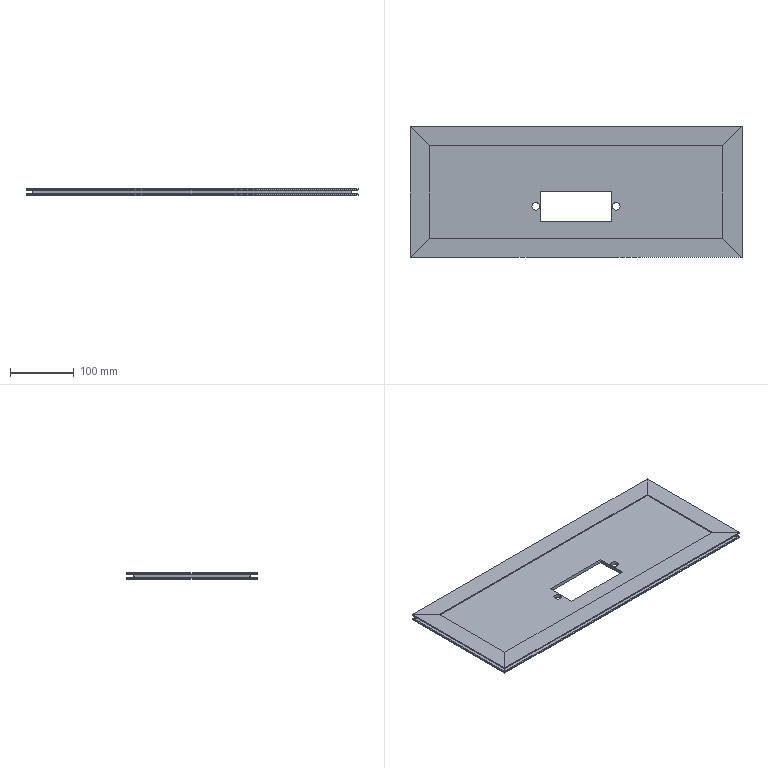Part | SolidWorks | features ICE 2, WeldMemberFeat 1, WeldmentFeature 1 | 5 solids | 102 faces | box 520 x 205 x 10 mm | volume 550676 mm3 | plane 82 | cylinder 20 | commonest cylinder face diameters 2 x16 12 x4